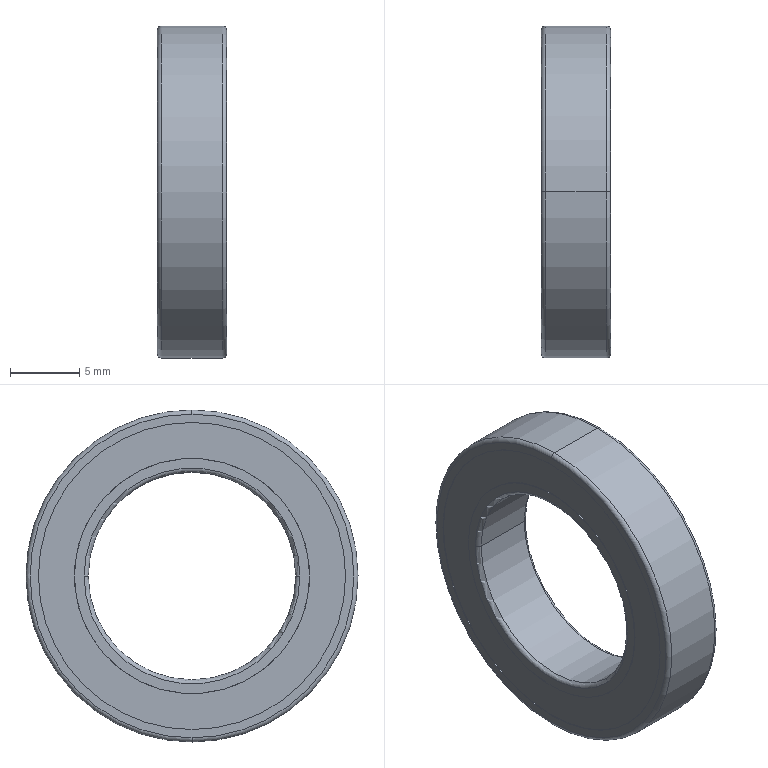Part | SolidWorks | features BaseBody 17 | 17 solids | 80 faces | box 5 x 24 x 24 mm | volume 921.616 mm3 | cylinder 28 | sphere 26 | torus 14 | plane 12 | commonest cylinder face diameters 17 x8 22.2 x8 17.75 x4 21.2 x4 15 x2 24 x2